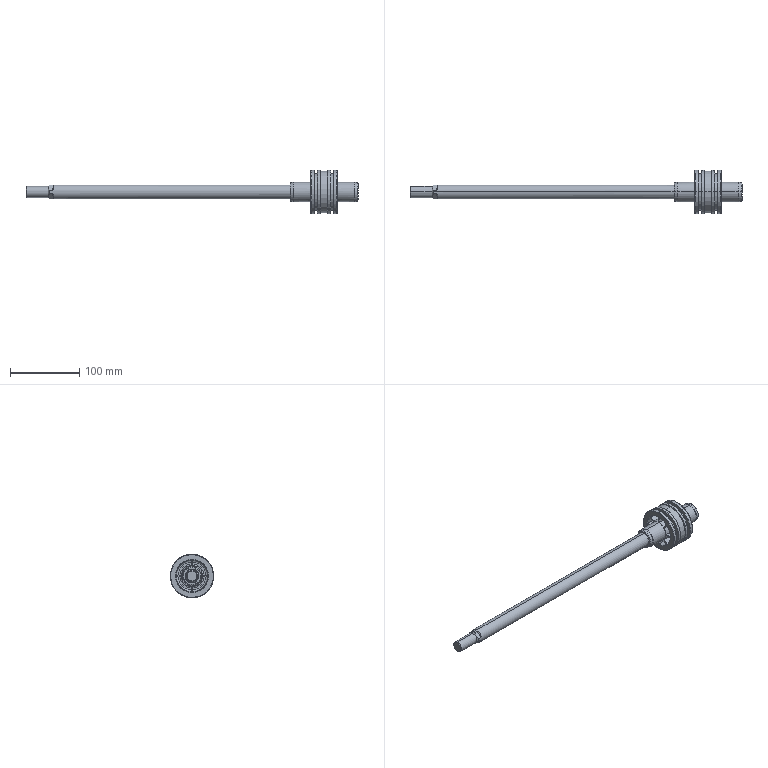Part | SolidWorks | features BaseBody 1 | 1 solid | 212 faces | box 478.5 x 62.5 x 62.5 mm | volume 216638 mm3 | cone 72 | plane 68 | spline 48 | cylinder 24 | commonest cylinder face diameters 62.5 x8 20 x4 28 x4 53 x4 16 x2 59.9 x2